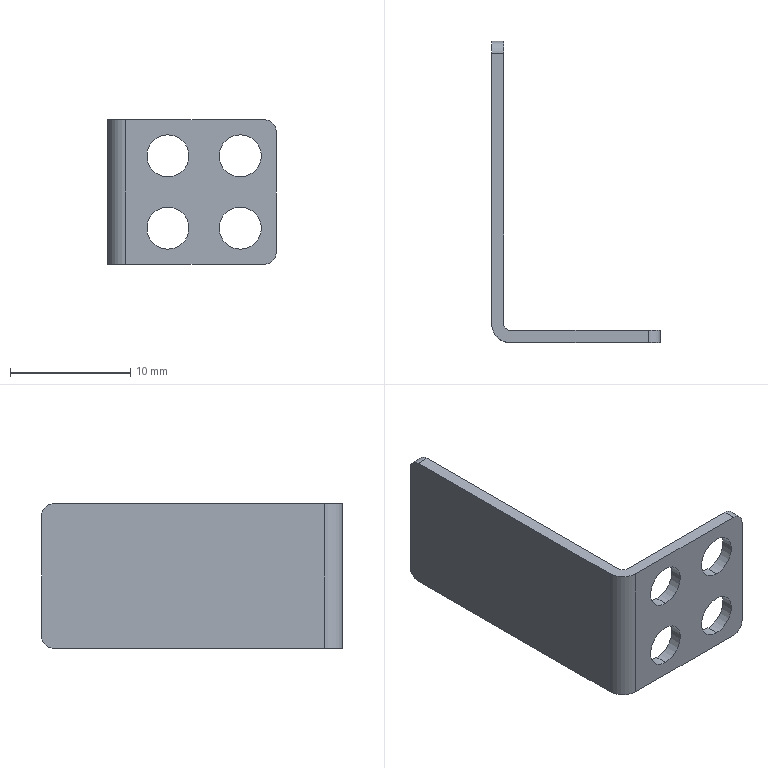Part | SolidWorks | features MoveFace 3, ICE 2, BaseBody 1, Fillet 1 | 1 solid | 22 faces | box 14 x 25 x 12 mm | volume 411.507 mm3 | cylinder 14 | plane 8 | commonest cylinder face diameters 3.5 x8 2 x4 1 x1 3 x1
STEP:
#1=CARTESIAN_POINT('',(4.,-12.5,-9.25));
#2=VERTEX_POINT('',#1);
#3=CARTESIAN_POINT('',(4.,-12.5,-12.75));
#4=VERTEX_POINT('',#3);
#5=CARTESIAN_POINT('',(4.,-12.5,-11.));
#6=DIRECTION('',(0.,-1.,0.));
#7=DIRECTION('',(0.,0.,-1.));
#8=AXIS2_PLACEMENT_3D('',#5,#6,#7);
#9=CIRCLE('',#8,1.75);
#10=EDGE_CURVE('',#2,#4,#9,.T.);
#11=ORIENTED_EDGE('',*,*,#10,.T.);
#12=CARTESIAN_POINT('',(4.,-11.5,-12.75));
#13=VERTEX_POINT('',#12);
#14=CARTESIAN_POINT('',(4.,-21.5,-12.75));
#15=DIRECTION('',(0.,1.,0.));
#16=VECTOR('',#15,1000.);
#17=LINE('',#14,#16);
#18=EDGE_CURVE('',#4,#13,#17,.T.);
#19=ORIENTED_EDGE('',*,*,#18,.T.);
#20=CARTESIAN_POINT('',(4.,-11.5,-9.25));
#21=VERTEX_POINT('',#20);
#22=CARTESIAN_POINT('',(4.,-11.5,-11.));
#23=DIRECTION('',(0.,1.,0.));
#24=DIRECTION('',(0.,0.,1.));
#25=AXIS2_PLACEMENT_3D('',#22,#23,#24);
#26=CIRCLE('',#25,1.75);
#27=EDGE_CURVE('',#13,#21,#26,.T.);
#28=ORIENTED_EDGE('',*,*,#27,.T.);
#29=CARTESIAN_POINT('',(4.,-21.5,-9.25));
#30=DIRECTION('',(0.,1.,0.));
#31=VECTOR('',#30,1000.);
#32=LINE('',#29,#31);
#33=EDGE_CURVE('',#2,#21,#32,.T.);
#34=ORIENTED_EDGE('',*,*,#33,.F.);
#35=EDGE_LOOP('',(#11,#19,#28,#34));
#36=FACE_OUTER_BOUND('',#35,.T.);
#37=CARTESIAN_POINT('',(4.,-21.5,-11.));
#38=DIRECTION('',(0.,1.,0.));
#39=DIRECTION('',(0.,0.,1.));
#40=AXIS2_PLACEMENT_3D('',#37,#38,#39);
#41=CYLINDRICAL_SURFACE('',#40,1.75);
#42=ADVANCED_FACE('',(#36),#41,.F.);
#43=CARTESIAN_POINT('',(-2.,-12.5,-12.75));
#44=VERTEX_POINT('',#43);
#45=CARTESIAN_POINT('',(-2.,-12.5,-9.25));
#46=VERTEX_POINT('',#45);
#47=CARTESIAN_POINT('',(-2.,-12.5,-11.));
#48=DIRECTION('',(0.,1.,0.));
#49=DIRECTION('',(0.,0.,1.));
#50=AXIS2_PLACEMENT_3D('',#47,#48,#49);
#51=CIRCLE('',#50,1.75);
#52=EDGE_CURVE('',#44,#46,#51,.T.);
#53=ORIENTED_EDGE('',*,*,#52,.F.);
#54=CARTESIAN_POINT('',(-2.,-11.5,-12.75));
#55=VERTEX_POINT('',#54);
#56=CARTESIAN_POINT('',(-2.,-11.5,-12.75));
#57=DIRECTION('',(0.,1.,0.));
#58=VECTOR('',#57,1000.);
#59=LINE('',#56,#58);
#60=EDGE_CURVE('',#44,#55,#59,.T.);
#61=ORIENTED_EDGE('',*,*,#60,.T.);
#62=CARTESIAN_POINT('',(-2.,-11.5,-9.25));
#63=VERTEX_POINT('',#62);
#64=CARTESIAN_POINT('',(-2.,-11.5,-11.));
#65=DIRECTION('',(0.,1.,0.));
#66=DIRECTION('',(0.,0.,1.));
#67=AXIS2_PLACEMENT_3D('',#64,#65,#66);
#68=CIRCLE('',#67,1.75);
#69=EDGE_CURVE('',#55,#63,#68,.T.);
#70=ORIENTED_EDGE('',*,*,#69,.T.);
#71=CARTESIAN_POINT('',(-2.,-11.5,-9.25));
#72=DIRECTION('',(0.,1.,0.));
#73=VECTOR('',#72,1000.);
#74=LINE('',#71,#73);
#75=EDGE_CURVE('',#46,#63,#74,.T.);
#76=ORIENTED_EDGE('',*,*,#75,.F.);
#77=EDGE_LOOP('',(#53,#61,#70,#76));
#78=FACE_OUTER_BOUND('',#77,.T.);
#79=CARTESIAN_POINT('',(-2.,-11.5,-11.));
#80=DIRECTION('',(0.,1.,0.));
#81=DIRECTION('',(0.,0.,1.));
#82=AXIS2_PLACEMENT_3D('',#79,#80,#81);
#83=CYLINDRICAL_SURFACE('',#82,1.75);
#84=ADVANCED_FACE('',(#78),#83,.F.);
#85=CARTESIAN_POINT('',(4.,-12.5,-6.75));
#86=VERTEX_POINT('',#85);
#87=CARTESIAN_POINT('',(4.,-12.5,-3.25));
#88=VERTEX_POINT('',#87);
#89=CARTESIAN_POINT('',(4.,-12.5,-5.));
#90=DIRECTION('',(0.,1.,0.));
#91=DIRECTION('',(0.,0.,1.));
#92=AXIS2_PLACEMENT_3D('',#89,#90,#91);
#93=CIRCLE('',#92,1.75);
#94=EDGE_CURVE('',#86,#88,#93,.T.);
#95=ORIENTED_EDGE('',*,*,#94,.F.);
#96=CARTESIAN_POINT('',(4.,-11.5,-6.75));
#97=VERTEX_POINT('',#96);
#98=CARTESIAN_POINT('',(4.,-11.5,-6.75));
#99=DIRECTION('',(0.,1.,0.));
#100=VECTOR('',#99,1000.);
#101=LINE('',#98,#100);
#102=EDGE_CURVE('',#86,#97,#101,.T.);
#103=ORIENTED_EDGE('',*,*,#102,.T.);
#104=CARTESIAN_POINT('',(4.,-11.5,-3.25));
#105=VERTEX_POINT('',#104);
#106=CARTESIAN_POINT('',(4.,-11.5,-5.));
#107=DIRECTION('',(0.,1.,0.));
#108=DIRECTION('',(0.,0.,1.));
#109=AXIS2_PLACEMENT_3D('',#106,#107,#108);
#110=CIRCLE('',#109,1.75);
#111=EDGE_CURVE('',#97,#105,#110,.T.);
#112=ORIENTED_EDGE('',*,*,#111,.T.);
#113=CARTESIAN_POINT('',(4.,-11.5,-3.25));
#114=DIRECTION('',(0.,1.,0.));
#115=VECTOR('',#114,1000.);
#116=LINE('',#113,#115);
#117=EDGE_CURVE('',#88,#105,#116,.T.);
#118=ORIENTED_EDGE('',*,*,#117,.F.);
#119=EDGE_LOOP('',(#95,#103,#112,#118));
#120=FACE_OUTER_BOUND('',#119,.T.);
#121=CARTESIAN_POINT('',(4.,-11.5,-5.));
#122=DIRECTION('',(0.,1.,0.));
#123=DIRECTION('',(0.,0.,1.));
#124=AXIS2_PLACEMENT_3D('',#121,#122,#123);
#125=CYLINDRICAL_SURFACE('',#124,1.75);
#126=ADVANCED_FACE('',(#120),#125,.F.);
#127=CARTESIAN_POINT('',(-2.,-12.5,-6.75));
#128=VERTEX_POINT('',#127);
#129=CARTESIAN_POINT('',(-2.,-12.5,-3.25));
#130=VERTEX_POINT('',#129);
#131=CARTESIAN_POINT('',(-2.,-12.5,-5.));
#132=DIRECTION('',(0.,1.,0.));
#133=DIRECTION('',(0.,0.,1.));
#134=AXIS2_PLACEMENT_3D('',#131,#132,#133);
#135=CIRCLE('',#134,1.75);
#136=EDGE_CURVE('',#128,#130,#135,.T.);
#137=ORIENTED_EDGE('',*,*,#136,.F.);
#138=CARTESIAN_POINT('',(-2.,-11.5,-6.75));
#139=VERTEX_POINT('',#138);
#140=CARTESIAN_POINT('',(-2.,-11.5,-6.75));
#141=DIRECTION('',(0.,1.,0.));
#142=VECTOR('',#141,1000.);
#143=LINE('',#140,#142);
#144=EDGE_CURVE('',#128,#139,#143,.T.);
#145=ORIENTED_EDGE('',*,*,#144,.T.);
#146=CARTESIAN_POINT('',(-2.,-11.5,-3.25));
#147=VERTEX_POINT('',#146);
#148=CARTESIAN_POINT('',(-2.,-11.5,-5.));
#149=DIRECTION('',(0.,1.,0.));
#150=DIRECTION('',(0.,0.,1.));
#151=AXIS2_PLACEMENT_3D('',#148,#149,#150);
#152=CIRCLE('',#151,1.75);
#153=EDGE_CURVE('',#139,#147,#152,.T.);
#154=ORIENTED_EDGE('',*,*,#153,.T.);
#155=CARTESIAN_POINT('',(-2.,-11.5,-3.25));
#156=DIRECTION('',(0.,1.,0.));
#157=VECTOR('',#156,1000.);
#158=LINE('',#155,#157);
#159=EDGE_CURVE('',#130,#147,#158,.T.);
#160=ORIENTED_EDGE('',*,*,#159,.F.);
#161=EDGE_LOOP('',(#137,#145,#154,#160));
#162=FACE_OUTER_BOUND('',#161,.T.);
#163=CARTESIAN_POINT('',(-2.,-11.5,-5.));
#164=DIRECTION('',(0.,1.,0.));
#165=DIRECTION('',(0.,0.,1.));
#166=AXIS2_PLACEMENT_3D('',#163,#164,#165);
#167=CYLINDRICAL_SURFACE('',#166,1.75);
#168=ADVANCED_FACE('',(#162),#167,.F.);
#169=CARTESIAN_POINT('',(-6.,12.5,-13.));
#170=VERTEX_POINT('',#169);
#171=CARTESIAN_POINT('',(-6.,11.5,-14.));
#172=VERTEX_POINT('',#171);
#173=CARTESIAN_POINT('',(-6.,11.5,-13.));
#174=DIRECTION('',(-1.,0.,0.));
#175=DIRECTION('',(0.,0.,-1.));
#176=AXIS2_PLACEMENT_3D('',#173,#174,#175);
#177=CIRCLE('',#176,1.);
#178=EDGE_CURVE('',#170,#172,#177,.T.);
#179=ORIENTED_EDGE('',*,*,#178,.F.);
#180=CARTESIAN_POINT('',(-6.,12.5,-3.));
#181=VERTEX_POINT('',#180);
#182=CARTESIAN_POINT('',(-6.,12.5,-15.));
#183=DIRECTION('',(0.,0.,-1.));
#184=VECTOR('',#183,1000.);
#185=LINE('',#182,#184);
#186=EDGE_CURVE('',#181,#170,#185,.T.);
#187=ORIENTED_EDGE('',*,*,#186,.F.);
#188=CARTESIAN_POINT('',(-6.,11.5,-2.));
#189=VERTEX_POINT('',#188);
#190=CARTESIAN_POINT('',(-6.,11.5,-3.));
#191=DIRECTION('',(-1.,0.,0.));
#192=DIRECTION('',(0.,0.,1.));
#193=AXIS2_PLACEMENT_3D('',#190,#191,#192);
#194=CIRCLE('',#193,1.);
#195=EDGE_CURVE('',#189,#181,#194,.T.);
#196=ORIENTED_EDGE('',*,*,#195,.F.);
#197=CARTESIAN_POINT('',(-6.,-11.,-2.));
#198=VERTEX_POINT('',#197);
#199=CARTESIAN_POINT('',(-6.,25.632,-2.));
#200=DIRECTION('',(0.,1.,0.));
#201=VECTOR('',#200,1000.);
#202=LINE('',#199,#201);
#203=EDGE_CURVE('',#198,#189,#202,.T.);
#204=ORIENTED_EDGE('',*,*,#203,.F.);
#205=CARTESIAN_POINT('',(-6.,-11.,-14.));
#206=VERTEX_POINT('',#205);
#207=CARTESIAN_POINT('',(-6.,-11.,-15.));
#208=DIRECTION('',(0.,0.,1.));
#209=VECTOR('',#208,1000.);
#210=LINE('',#207,#209);
#211=EDGE_CURVE('',#206,#198,#210,.T.);
#212=ORIENTED_EDGE('',*,*,#211,.F.);
#213=CARTESIAN_POINT('',(-6.,25.632,-14.));
#214=DIRECTION('',(0.,-1.,0.));
#215=VECTOR('',#214,1000.);
#216=LINE('',#213,#215);
#217=EDGE_CURVE('',#172,#206,#216,.T.);
#218=ORIENTED_EDGE('',*,*,#217,.F.);
#219=EDGE_LOOP('',(#179,#187,#196,#204,#212,#218));
#220=FACE_OUTER_BOUND('',#219,.T.);
#221=CARTESIAN_POINT('',(-6.,25.632,-15.));
#222=DIRECTION('',(-1.,0.,0.));
#223=DIRECTION('',(0.,-1.,0.));
#224=AXIS2_PLACEMENT_3D('',#221,#222,#223);
#225=PLANE('',#224);
#226=ADVANCED_FACE('',(#220),#225,.F.);
#227=CARTESIAN_POINT('',(-5.5,-11.5,-14.));
#228=VERTEX_POINT('',#227);
#229=CARTESIAN_POINT('',(6.,-11.5,-14.));
#230=VERTEX_POINT('',#229);
#231=CARTESIAN_POINT('',(28.84,-11.5,-14.));
#232=DIRECTION('',(1.,0.,0.));
#233=VECTOR('',#232,1000.);
#234=LINE('',#231,#233);
#235=EDGE_CURVE('',#228,#230,#234,.T.);
#236=ORIENTED_EDGE('',*,*,#235,.T.);
#237=CARTESIAN_POINT('',(6.,-12.5,-14.));
#238=VERTEX_POINT('',#237);
#239=CARTESIAN_POINT('',(6.,-12.5,-14.));
#240=DIRECTION('',(0.,-1.,0.));
#241=VECTOR('',#240,1000.);
#242=LINE('',#239,#241);
#243=EDGE_CURVE('',#230,#238,#242,.T.);
#244=ORIENTED_EDGE('',*,*,#243,.T.);
#245=CARTESIAN_POINT('',(-5.5,-12.5,-14.));
#246=VERTEX_POINT('',#245);
#247=CARTESIAN_POINT('',(-7.,-12.5,-14.));
#248=DIRECTION('',(1.,0.,0.));
#249=VECTOR('',#248,1000.);
#250=LINE('',#247,#249);
#251=EDGE_CURVE('',#246,#238,#250,.T.);
#252=ORIENTED_EDGE('',*,*,#251,.F.);
#253=CARTESIAN_POINT('',(-7.,-11.,-14.));
#254=VERTEX_POINT('',#253);
#255=CARTESIAN_POINT('',(-5.5,-11.,-14.));
#256=DIRECTION('',(0.,0.,1.));
#257=DIRECTION('',(1.,0.,0.));
#258=AXIS2_PLACEMENT_3D('',#255,#256,#257);
#259=CIRCLE('',#258,1.5);
#260=EDGE_CURVE('',#254,#246,#259,.T.);
#261=ORIENTED_EDGE('',*,*,#260,.F.);
#262=CARTESIAN_POINT('',(-7.,11.5,-14.));
#263=VERTEX_POINT('',#262);
#264=CARTESIAN_POINT('',(-7.,12.5,-14.));
#265=DIRECTION('',(0.,-1.,0.));
#266=VECTOR('',#265,1000.);
#267=LINE('',#264,#266);
#268=EDGE_CURVE('',#263,#254,#267,.T.);
#269=ORIENTED_EDGE('',*,*,#268,.F.);
#270=CARTESIAN_POINT('',(-5.,11.5,-14.));
#271=DIRECTION('',(-1.,0.,0.));
#272=VECTOR('',#271,1000.);
#273=LINE('',#270,#272);
#274=EDGE_CURVE('',#172,#263,#273,.T.);
#275=ORIENTED_EDGE('',*,*,#274,.F.);
#276=ORIENTED_EDGE('',*,*,#217,.T.);
#277=CARTESIAN_POINT('',(-5.5,-11.,-14.));
#278=DIRECTION('',(0.,0.,-1.));
#279=DIRECTION('',(-1.,0.,0.));
#280=AXIS2_PLACEMENT_3D('',#277,#278,#279);
#281=CIRCLE('',#280,0.5);
#282=EDGE_CURVE('',#228,#206,#281,.T.);
#283=ORIENTED_EDGE('',*,*,#282,.F.);
#284=EDGE_LOOP('',(#236,#244,#252,#261,#269,#275,#276,#283));
#285=FACE_OUTER_BOUND('',#284,.T.);
#286=CARTESIAN_POINT('',(-5.,12.5,-14.));
#287=DIRECTION('',(0.,0.,1.));
#288=DIRECTION('',(1.,0.,0.));
#289=AXIS2_PLACEMENT_3D('',#286,#287,#288);
#290=PLANE('',#289);
#291=ADVANCED_FACE('',(#285),#290,.F.);
#292=CARTESIAN_POINT('',(-7.,12.5,-13.));
#293=VERTEX_POINT('',#292);
#294=CARTESIAN_POINT('',(-7.,11.5,-13.));
#295=DIRECTION('',(1.,0.,0.));
#296=DIRECTION('',(0.,0.,-1.));
#297=AXIS2_PLACEMENT_3D('',#294,#295,#296);
#298=CIRCLE('',#297,1.);
#299=EDGE_CURVE('',#263,#293,#298,.T.);
#300=ORIENTED_EDGE('',*,*,#299,.T.);
#301=CARTESIAN_POINT('',(-7.,12.5,-13.));
#302=DIRECTION('',(1.,0.,0.));
#303=VECTOR('',#302,1000.);
#304=LINE('',#301,#303);
#305=EDGE_CURVE('',#293,#170,#304,.T.);
#306=ORIENTED_EDGE('',*,*,#305,.T.);
#307=ORIENTED_EDGE('',*,*,#178,.T.);
#308=ORIENTED_EDGE('',*,*,#274,.T.);
#309=EDGE_LOOP('',(#300,#306,#307,#308));
#310=FACE_OUTER_BOUND('',#309,.T.);
#311=CARTESIAN_POINT('',(-7.,11.5,-13.));
#312=DIRECTION('',(1.,0.,0.));
#313=DIRECTION('',(0.,0.,-1.));
#314=AXIS2_PLACEMENT_3D('',#311,#312,#313);
#315=CYLINDRICAL_SURFACE('',#314,1.);
#316=ADVANCED_FACE('',(#310),#315,.T.);
#317=CARTESIAN_POINT('',(-7.,12.5,-3.));
#318=VERTEX_POINT('',#317);
#319=CARTESIAN_POINT('',(-7.,12.5,-15.));
#320=DIRECTION('',(0.,0.,1.));
#321=VECTOR('',#320,1000.);
#322=LINE('',#319,#321);
#323=EDGE_CURVE('',#293,#318,#322,.T.);
#324=ORIENTED_EDGE('',*,*,#323,.T.);
#325=CARTESIAN_POINT('',(-7.,12.5,-3.));
#326=DIRECTION('',(1.,0.,0.));
#327=VECTOR('',#326,1000.);
#328=LINE('',#325,#327);
#329=EDGE_CURVE('',#318,#181,#328,.T.);
#330=ORIENTED_EDGE('',*,*,#329,.T.);
#331=ORIENTED_EDGE('',*,*,#186,.T.);
#332=ORIENTED_EDGE('',*,*,#305,.F.);
#333=EDGE_LOOP('',(#324,#330,#331,#332));
#334=FACE_OUTER_BOUND('',#333,.T.);
#335=CARTESIAN_POINT('',(-7.,12.5,-15.));
#336=DIRECTION('',(0.,1.,0.));
#337=DIRECTION('',(0.,0.,1.));
#338=AXIS2_PLACEMENT_3D('',#335,#336,#337);
#339=PLANE('',#338);
#340=ADVANCED_FACE('',(#334),#339,.T.);
#341=CARTESIAN_POINT('',(-7.,11.5,-2.));
#342=VERTEX_POINT('',#341);
#343=CARTESIAN_POINT('',(-7.,11.5,-3.));
#344=DIRECTION('',(1.,0.,0.));
#345=DIRECTION('',(0.,0.,1.));
#346=AXIS2_PLACEMENT_3D('',#343,#344,#345);
#347=CIRCLE('',#346,1.);
#348=EDGE_CURVE('',#318,#342,#347,.T.);
#349=ORIENTED_EDGE('',*,*,#348,.T.);
#350=CARTESIAN_POINT('',(0.,11.5,-2.));
#351=DIRECTION('',(1.,0.,0.));
#352=VECTOR('',#351,1000.);
#353=LINE('',#350,#352);
#354=EDGE_CURVE('',#342,#189,#353,.T.);
#355=ORIENTED_EDGE('',*,*,#354,.T.);
#356=ORIENTED_EDGE('',*,*,#195,.T.);
#357=ORIENTED_EDGE('',*,*,#329,.F.);
#358=EDGE_LOOP('',(#349,#355,#356,#357));
#359=FACE_OUTER_BOUND('',#358,.T.);
#360=CARTESIAN_POINT('',(0.,11.5,-3.));
#361=DIRECTION('',(-1.,0.,0.));
#362=DIRECTION('',(0.,0.,1.));
#363=AXIS2_PLACEMENT_3D('',#360,#361,#362);
#364=CYLINDRICAL_SURFACE('',#363,1.);
#365=ADVANCED_FACE('',(#359),#364,.T.);
#366=CARTESIAN_POINT('',(6.,-11.5,-2.));
#367=VERTEX_POINT('',#366);
#368=CARTESIAN_POINT('',(-5.5,-11.5,-2.));
#369=VERTEX_POINT('',#368);
#370=CARTESIAN_POINT('',(0.,-11.5,-2.));
#371=DIRECTION('',(-1.,0.,0.));
#372=VECTOR('',#371,1000.);
#373=LINE('',#370,#372);
#374=EDGE_CURVE('',#367,#369,#373,.T.);
#375=ORIENTED_EDGE('',*,*,#374,.T.);
#376=CARTESIAN_POINT('',(-5.5,-11.,-2.));
#377=DIRECTION('',(0.,0.,-1.));
#378=DIRECTION('',(-1.,0.,0.));
#379=AXIS2_PLACEMENT_3D('',#376,#377,#378);
#380=CIRCLE('',#379,0.5);
#381=EDGE_CURVE('',#369,#198,#380,.T.);
#382=ORIENTED_EDGE('',*,*,#381,.T.);
#383=ORIENTED_EDGE('',*,*,#203,.T.);
#384=ORIENTED_EDGE('',*,*,#354,.F.);
#385=CARTESIAN_POINT('',(-7.,-11.,-2.));
#386=VERTEX_POINT('',#385);
#387=CARTESIAN_POINT('',(-7.,0.,-2.));
#388=DIRECTION('',(0.,-1.,0.));
#389=VECTOR('',#388,1000.);
#390=LINE('',#387,#389);
#391=EDGE_CURVE('',#342,#386,#390,.T.);
#392=ORIENTED_EDGE('',*,*,#391,.T.);
#393=CARTESIAN_POINT('',(-5.5,-12.5,-2.));
#394=VERTEX_POINT('',#393);
#395=CARTESIAN_POINT('',(-5.5,-11.,-2.));
#396=DIRECTION('',(0.,0.,1.));
#397=DIRECTION('',(1.,0.,0.));
#398=AXIS2_PLACEMENT_3D('',#395,#396,#397);
#399=CIRCLE('',#398,1.5);
#400=EDGE_CURVE('',#386,#394,#399,.T.);
#401=ORIENTED_EDGE('',*,*,#400,.T.);
#402=CARTESIAN_POINT('',(6.,-12.5,-2.));
#403=VERTEX_POINT('',#402);
#404=CARTESIAN_POINT('',(0.,-12.5,-2.));
#405=DIRECTION('',(1.,0.,0.));
#406=VECTOR('',#405,1000.);
#407=LINE('',#404,#406);
#408=EDGE_CURVE('',#394,#403,#407,.T.);
#409=ORIENTED_EDGE('',*,*,#408,.T.);
#410=CARTESIAN_POINT('',(6.,0.,-2.));
#411=DIRECTION('',(0.,1.,0.));
#412=VECTOR('',#411,1000.);
#413=LINE('',#410,#412);
#414=EDGE_CURVE('',#403,#367,#413,.T.);
#415=ORIENTED_EDGE('',*,*,#414,.T.);
#416=EDGE_LOOP('',(#375,#382,#383,#384,#392,#401,#409,#415));
#417=FACE_OUTER_BOUND('',#416,.T.);
#418=CARTESIAN_POINT('',(0.,0.,-2.));
#419=DIRECTION('',(0.,0.,1.));
#420=DIRECTION('',(1.,0.,0.));
#421=AXIS2_PLACEMENT_3D('',#418,#419,#420);
#422=PLANE('',#421);
#423=ADVANCED_FACE('',(#417),#422,.T.);
#424=ORIENTED_EDGE('',*,*,#282,.T.);
#425=ORIENTED_EDGE('',*,*,#211,.T.);
#426=ORIENTED_EDGE('',*,*,#381,.F.);
#427=CARTESIAN_POINT('',(-5.5,-11.5,-15.));
#428=DIRECTION('',(0.,0.,1.));
#429=VECTOR('',#428,1000.);
#430=LINE('',#427,#429);
#431=EDGE_CURVE('',#228,#369,#430,.T.);
#432=ORIENTED_EDGE('',*,*,#431,.F.);
#433=EDGE_LOOP('',(#424,#425,#426,#432));
#434=FACE_OUTER_BOUND('',#433,.T.);
#435=CARTESIAN_POINT('',(-5.5,-11.,-15.));
#436=DIRECTION('',(0.,0.,-1.));
#437=DIRECTION('',(-1.,0.,0.));
#438=AXIS2_PLACEMENT_3D('',#435,#436,#437);
#439=CYLINDRICAL_SURFACE('',#438,0.5);
#440=ADVANCED_FACE('',(#434),#439,.F.);
#441=ORIENTED_EDGE('',*,*,#391,.F.);
#442=ORIENTED_EDGE('',*,*,#348,.F.);
#443=ORIENTED_EDGE('',*,*,#323,.F.);
#444=ORIENTED_EDGE('',*,*,#299,.F.);
#445=ORIENTED_EDGE('',*,*,#268,.T.);
#446=CARTESIAN_POINT('',(-7.,-11.,-15.));
#447=DIRECTION('',(0.,0.,1.));
#448=VECTOR('',#447,1000.);
#449=LINE('',#446,#448);
#450=EDGE_CURVE('',#254,#386,#449,.T.);
#451=ORIENTED_EDGE('',*,*,#450,.T.);
#452=EDGE_LOOP('',(#441,#442,#443,#444,#445,#451));
#453=FACE_OUTER_BOUND('',#452,.T.);
#454=CARTESIAN_POINT('',(-7.,12.5,-15.));
#455=DIRECTION('',(-1.,0.,0.));
#456=DIRECTION('',(0.,-1.,0.));
#457=AXIS2_PLACEMENT_3D('',#454,#455,#456);
#458=PLANE('',#457);
#459=ADVANCED_FACE('',(#453),#458,.T.);
#460=ORIENTED_EDGE('',*,*,#400,.F.);
#461=ORIENTED_EDGE('',*,*,#450,.F.);
#462=ORIENTED_EDGE('',*,*,#260,.T.);
#463=CARTESIAN_POINT('',(-5.5,-12.5,-15.));
#464=DIRECTION('',(0.,0.,1.));
#465=VECTOR('',#464,1000.);
#466=LINE('',#463,#465);
#467=EDGE_CURVE('',#246,#394,#466,.T.);
#468=ORIENTED_EDGE('',*,*,#467,.T.);
#469=EDGE_LOOP('',(#460,#461,#462,#468));
#470=FACE_OUTER_BOUND('',#469,.T.);
#471=CARTESIAN_POINT('',(-5.5,-11.,-15.));
#472=DIRECTION('',(0.,0.,1.));
#473=DIRECTION('',(1.,0.,0.));
#474=AXIS2_PLACEMENT_3D('',#471,#472,#473);
#475=CYLINDRICAL_SURFACE('',#474,1.5);
#476=ADVANCED_FACE('',(#470),#475,.T.);
#477=CARTESIAN_POINT('',(4.,-11.5,-11.));
#478=DIRECTION('',(0.,1.,0.));
#479=DIRECTION('',(0.,0.,1.));
#480=AXIS2_PLACEMENT_3D('',#477,#478,#479);
#481=CIRCLE('',#480,1.75);
#482=EDGE_CURVE('',#21,#13,#481,.T.);
#483=ORIENTED_EDGE('',*,*,#482,.F.);
#484=ORIENTED_EDGE('',*,*,#27,.F.);
#485=EDGE_LOOP('',(#483,#484));
#486=FACE_BOUND('',#485,.T.);
#487=CARTESIAN_POINT('',(7.,-11.5,-13.));
#488=VERTEX_POINT('',#487);
#489=CARTESIAN_POINT('',(7.,-11.5,-3.));
#490=VERTEX_POINT('',#489);
#491=CARTESIAN_POINT('',(7.,-11.5,-15.));
#492=DIRECTION('',(0.,0.,1.));
#493=VECTOR('',#492,1000.);
#494=LINE('',#491,#493);
#495=EDGE_CURVE('',#488,#490,#494,.T.);
#496=ORIENTED_EDGE('',*,*,#495,.F.);
#497=CARTESIAN_POINT('',(6.,-11.5,-13.));
#498=DIRECTION('',(0.,1.,0.));
#499=DIRECTION('',(0.,0.,-1.));
#500=AXIS2_PLACEMENT_3D('',#497,#498,#499);
#501=CIRCLE('',#500,1.);
#502=EDGE_CURVE('',#488,#230,#501,.T.);
#503=ORIENTED_EDGE('',*,*,#502,.T.);
#504=ORIENTED_EDGE('',*,*,#235,.F.);
#505=ORIENTED_EDGE('',*,*,#431,.T.);
#506=ORIENTED_EDGE('',*,*,#374,.F.);
#507=CARTESIAN_POINT('',(6.,-11.5,-3.));
#508=DIRECTION('',(0.,-1.,0.));
#509=DIRECTION('',(-1.,0.,0.));
#510=AXIS2_PLACEMENT_3D('',#507,#508,#509);
#511=CIRCLE('',#510,1.);
#512=EDGE_CURVE('',#490,#367,#511,.T.);
#513=ORIENTED_EDGE('',*,*,#512,.F.);
#514=EDGE_LOOP('',(#496,#503,#504,#505,#506,#513));
#515=FACE_OUTER_BOUND('',#514,.T.);
#516=CARTESIAN_POINT('',(-2.,-11.5,-11.));
#517=DIRECTION('',(0.,1.,0.));
#518=DIRECTION('',(0.,0.,1.));
#519=AXIS2_PLACEMENT_3D('',#516,#517,#518);
#520=CIRCLE('',#519,1.75);
#521=EDGE_CURVE('',#63,#55,#520,.T.);
#522=ORIENTED_EDGE('',*,*,#521,.F.);
#523=ORIENTED_EDGE('',*,*,#69,.F.);
#524=EDGE_LOOP('',(#522,#523));
#525=FACE_BOUND('',#524,.T.);
#526=CARTESIAN_POINT('',(4.,-11.5,-5.));
#527=DIRECTION('',(0.,1.,0.));
#528=DIRECTION('',(0.,0.,1.));
#529=AXIS2_PLACEMENT_3D('',#526,#527,#528);
#530=CIRCLE('',#529,1.75);
#531=EDGE_CURVE('',#105,#97,#530,.T.);
#532=ORIENTED_EDGE('',*,*,#531,.F.);
#533=ORIENTED_EDGE('',*,*,#111,.F.);
#534=EDGE_LOOP('',(#532,#533));
#535=FACE_BOUND('',#534,.T.);
#536=CARTESIAN_POINT('',(-2.,-11.5,-5.));
#537=DIRECTION('',(0.,1.,0.));
#538=DIRECTION('',(0.,0.,1.));
#539=AXIS2_PLACEMENT_3D('',#536,#537,#538);
#540=CIRCLE('',#539,1.75);
#541=EDGE_CURVE('',#147,#139,#540,.T.);
#542=ORIENTED_EDGE('',*,*,#541,.F.);
#543=ORIENTED_EDGE('',*,*,#153,.F.);
#544=EDGE_LOOP('',(#542,#543));
#545=FACE_BOUND('',#544,.T.);
#546=CARTESIAN_POINT('',(28.84,-11.5,-15.));
#547=DIRECTION('',(0.,-1.,0.));
#548=DIRECTION('',(0.,0.,-1.));
#549=AXIS2_PLACEMENT_3D('',#546,#547,#548);
#550=PLANE('',#549);
#551=ADVANCED_FACE('',(#486,#515,#525,#535,#545),#550,.F.);
#552=ORIENTED_EDGE('',*,*,#512,.T.);
#553=ORIENTED_EDGE('',*,*,#414,.F.);
#554=CARTESIAN_POINT('',(7.,-12.5,-3.));
#555=VERTEX_POINT('',#554);
#556=CARTESIAN_POINT('',(6.,-12.5,-3.));
#557=DIRECTION('',(0.,1.,0.));
#558=DIRECTION('',(-1.,0.,0.));
#559=AXIS2_PLACEMENT_3D('',#556,#557,#558);
#560=CIRCLE('',#559,1.);
#561=EDGE_CURVE('',#403,#555,#560,.T.);
#562=ORIENTED_EDGE('',*,*,#561,.T.);
#563=CARTESIAN_POINT('',(7.,0.,-3.));
#564=DIRECTION('',(0.,1.,0.));
#565=VECTOR('',#564,1000.);
#566=LINE('',#563,#565);
#567=EDGE_CURVE('',#555,#490,#566,.T.);
#568=ORIENTED_EDGE('',*,*,#567,.T.);
#569=EDGE_LOOP('',(#552,#553,#562,#568));
#570=FACE_OUTER_BOUND('',#569,.T.);
#571=CARTESIAN_POINT('',(6.,0.,-3.));
#572=DIRECTION('',(0.,1.,0.));
#573=DIRECTION('',(-1.,0.,0.));
#574=AXIS2_PLACEMENT_3D('',#571,#572,#573);
#575=CYLINDRICAL_SURFACE('',#574,1.);
#576=ADVANCED_FACE('',(#570),#575,.T.);
#577=ORIENTED_EDGE('',*,*,#251,.T.);
#578=CARTESIAN_POINT('',(7.,-12.5,-13.));
#579=VERTEX_POINT('',#578);
#580=CARTESIAN_POINT('',(6.,-12.5,-13.));
#581=DIRECTION('',(0.,-1.,0.));
#582=DIRECTION('',(0.,0.,-1.));
#583=AXIS2_PLACEMENT_3D('',#580,#581,#582);
#584=CIRCLE('',#583,1.);
#585=EDGE_CURVE('',#238,#579,#584,.T.);
#586=ORIENTED_EDGE('',*,*,#585,.T.);
#587=CARTESIAN_POINT('',(7.,-12.5,-15.));
#588=DIRECTION('',(0.,0.,1.));
#589=VECTOR('',#588,1000.);
#590=LINE('',#587,#589);
#591=EDGE_CURVE('',#579,#555,#590,.T.);
#592=ORIENTED_EDGE('',*,*,#591,.T.);
#593=ORIENTED_EDGE('',*,*,#561,.F.);
#594=ORIENTED_EDGE('',*,*,#408,.F.);
#595=ORIENTED_EDGE('',*,*,#467,.F.);
#596=EDGE_LOOP('',(#577,#586,#592,#593,#594,#595));
#597=FACE_OUTER_BOUND('',#596,.T.);
#598=ORIENTED_EDGE('',*,*,#10,.F.);
#599=CARTESIAN_POINT('',(4.,-12.5,-11.));
#600=DIRECTION('',(0.,-1.,0.));
#601=DIRECTION('',(0.,0.,-1.));
#602=AXIS2_PLACEMENT_3D('',#599,#600,#601);
#603=CIRCLE('',#602,1.75);
#604=EDGE_CURVE('',#4,#2,#603,.T.);
#605=ORIENTED_EDGE('',*,*,#604,.F.);
#606=EDGE_LOOP('',(#598,#605));
#607=FACE_BOUND('',#606,.T.);
#608=CARTESIAN_POINT('',(-2.,-12.5,-11.));
#609=DIRECTION('',(0.,1.,0.));
#610=DIRECTION('',(0.,0.,1.));
#611=AXIS2_PLACEMENT_3D('',#608,#609,#610);
#612=CIRCLE('',#611,1.75);
#613=EDGE_CURVE('',#46,#44,#612,.T.);
#614=ORIENTED_EDGE('',*,*,#613,.T.);
#615=ORIENTED_EDGE('',*,*,#52,.T.);
#616=EDGE_LOOP('',(#614,#615));
#617=FACE_BOUND('',#616,.T.);
#618=CARTESIAN_POINT('',(4.,-12.5,-5.));
#619=DIRECTION('',(0.,1.,0.));
#620=DIRECTION('',(0.,0.,1.));
#621=AXIS2_PLACEMENT_3D('',#618,#619,#620);
#622=CIRCLE('',#621,1.75);
#623=EDGE_CURVE('',#88,#86,#622,.T.);
#624=ORIENTED_EDGE('',*,*,#623,.T.);
#625=ORIENTED_EDGE('',*,*,#94,.T.);
#626=EDGE_LOOP('',(#624,#625));
#627=FACE_BOUND('',#626,.T.);
#628=CARTESIAN_POINT('',(-2.,-12.5,-5.));
#629=DIRECTION('',(0.,1.,0.));
#630=DIRECTION('',(0.,0.,1.));
#631=AXIS2_PLACEMENT_3D('',#628,#629,#630);
#632=CIRCLE('',#631,1.75);
#633=EDGE_CURVE('',#130,#128,#632,.T.);
#634=ORIENTED_EDGE('',*,*,#633,.T.);
#635=ORIENTED_EDGE('',*,*,#136,.T.);
#636=EDGE_LOOP('',(#634,#635));
#637=FACE_BOUND('',#636,.T.);
#638=CARTESIAN_POINT('',(-7.,-12.5,-15.));
#639=DIRECTION('',(0.,-1.,0.));
#640=DIRECTION('',(0.,0.,-1.));
#641=AXIS2_PLACEMENT_3D('',#638,#639,#640);
#642=PLANE('',#641);
#643=ADVANCED_FACE('',(#597,#607,#617,#627,#637),#642,.T.);
#644=ORIENTED_EDGE('',*,*,#591,.F.);
#645=CARTESIAN_POINT('',(7.,-11.5,-13.));
#646=DIRECTION('',(0.,1.,0.));
#647=VECTOR('',#646,1000.);
#648=LINE('',#645,#647);
#649=EDGE_CURVE('',#579,#488,#648,.T.);
#650=ORIENTED_EDGE('',*,*,#649,.T.);
#651=ORIENTED_EDGE('',*,*,#495,.T.);
#652=ORIENTED_EDGE('',*,*,#567,.F.);
#653=EDGE_LOOP('',(#644,#650,#651,#652));
#654=FACE_OUTER_BOUND('',#653,.T.);
#655=CARTESIAN_POINT('',(7.,12.5,-15.));
#656=DIRECTION('',(1.,0.,0.));
#657=DIRECTION('',(0.,1.,0.));
#658=AXIS2_PLACEMENT_3D('',#655,#656,#657);
#659=PLANE('',#658);
#660=ADVANCED_FACE('',(#654),#659,.T.);
#661=ORIENTED_EDGE('',*,*,#60,.F.);
#662=ORIENTED_EDGE('',*,*,#613,.F.);
#663=ORIENTED_EDGE('',*,*,#75,.T.);
#664=ORIENTED_EDGE('',*,*,#521,.T.);
#665=EDGE_LOOP('',(#661,#662,#663,#664));
#666=FACE_OUTER_BOUND('',#665,.T.);
#667=CARTESIAN_POINT('',(-2.,-11.5,-11.));
#668=DIRECTION('',(0.,1.,0.));
#669=DIRECTION('',(0.,0.,1.));
#670=AXIS2_PLACEMENT_3D('',#667,#668,#669);
#671=CYLINDRICAL_SURFACE('',#670,1.75);
#672=ADVANCED_FACE('',(#666),#671,.F.);
#673=ORIENTED_EDGE('',*,*,#102,.F.);
#674=ORIENTED_EDGE('',*,*,#623,.F.);
#675=ORIENTED_EDGE('',*,*,#117,.T.);
#676=ORIENTED_EDGE('',*,*,#531,.T.);
#677=EDGE_LOOP('',(#673,#674,#675,#676));
#678=FACE_OUTER_BOUND('',#677,.T.);
#679=CARTESIAN_POINT('',(4.,-11.5,-5.));
#680=DIRECTION('',(0.,1.,0.));
#681=DIRECTION('',(0.,0.,1.));
#682=AXIS2_PLACEMENT_3D('',#679,#680,#681);
#683=CYLINDRICAL_SURFACE('',#682,1.75);
#684=ADVANCED_FACE('',(#678),#683,.F.);
#685=ORIENTED_EDGE('',*,*,#144,.F.);
#686=ORIENTED_EDGE('',*,*,#633,.F.);
#687=ORIENTED_EDGE('',*,*,#159,.T.);
#688=ORIENTED_EDGE('',*,*,#541,.T.);
#689=EDGE_LOOP('',(#685,#686,#687,#688));
#690=FACE_OUTER_BOUND('',#689,.T.);
#691=CARTESIAN_POINT('',(-2.,-11.5,-5.));
#692=DIRECTION('',(0.,1.,0.));
#693=DIRECTION('',(0.,0.,1.));
#694=AXIS2_PLACEMENT_3D('',#691,#692,#693);
#695=CYLINDRICAL_SURFACE('',#694,1.75);
#696=ADVANCED_FACE('',(#690),#695,.F.);
#697=ORIENTED_EDGE('',*,*,#18,.F.);
#698=ORIENTED_EDGE('',*,*,#604,.T.);
#699=ORIENTED_EDGE('',*,*,#33,.T.);
#700=ORIENTED_EDGE('',*,*,#482,.T.);
#701=EDGE_LOOP('',(#697,#698,#699,#700));
#702=FACE_OUTER_BOUND('',#701,.T.);
#703=CARTESIAN_POINT('',(4.,-21.5,-11.));
#704=DIRECTION('',(0.,1.,0.));
#705=DIRECTION('',(0.,0.,1.));
#706=AXIS2_PLACEMENT_3D('',#703,#704,#705);
#707=CYLINDRICAL_SURFACE('',#706,1.75);
#708=ADVANCED_FACE('',(#702),#707,.F.);
#709=ORIENTED_EDGE('',*,*,#502,.F.);
#710=ORIENTED_EDGE('',*,*,#649,.F.);
#711=ORIENTED_EDGE('',*,*,#585,.F.);
#712=ORIENTED_EDGE('',*,*,#243,.F.);
#713=EDGE_LOOP('',(#709,#710,#711,#712));
#714=FACE_OUTER_BOUND('',#713,.T.);
#715=CARTESIAN_POINT('',(6.,12.5,-13.));
#716=DIRECTION('',(0.,1.,0.));
#717=DIRECTION('',(-1.,0.,0.));
#718=AXIS2_PLACEMENT_3D('',#715,#716,#717);
#719=CYLINDRICAL_SURFACE('',#718,1.);
#720=ADVANCED_FACE('',(#714),#719,.T.);
#721=CLOSED_SHELL('',(#42,#84,#126,#168,#226,#291,#316,#340,#365,#423,#440,#459,#476,#551,#576,#643,#660,#672,#684,#696,#708,#720));
#722=MANIFOLD_SOLID_BREP('',#721);
#723=CARTESIAN_POINT('',(0.,0.,0.));
#724=DIRECTION('',(0.,0.,1.));
#725=DIRECTION('',(1.,0.,0.));
#726=AXIS2_PLACEMENT_3D('',#723,#724,#725);
#727=(LENGTH_UNIT()NAMED_UNIT(*)SI_UNIT(.MILLI.,.METRE.));
#728=UNCERTAINTY_MEASURE_WITH_UNIT(LENGTH_MEASURE(0.00001),#727,'','');
#729=(NAMED_UNIT(*)PLANE_ANGLE_UNIT()SI_UNIT($,.RADIAN.));
#730=(NAMED_UNIT(*)SI_UNIT($,.STERADIAN.)SOLID_ANGLE_UNIT());
#731=(GEOMETRIC_REPRESENTATION_CONTEXT(3)GLOBAL_UNCERTAINTY_ASSIGNED_CONTEXT((#728))GLOBAL_UNIT_ASSIGNED_CONTEXT((#727,#729,#730))REPRESENTATION_CONTEXT('',''));
#732=ADVANCED_BREP_SHAPE_REPRESENTATION('',(#722,#726),#731);